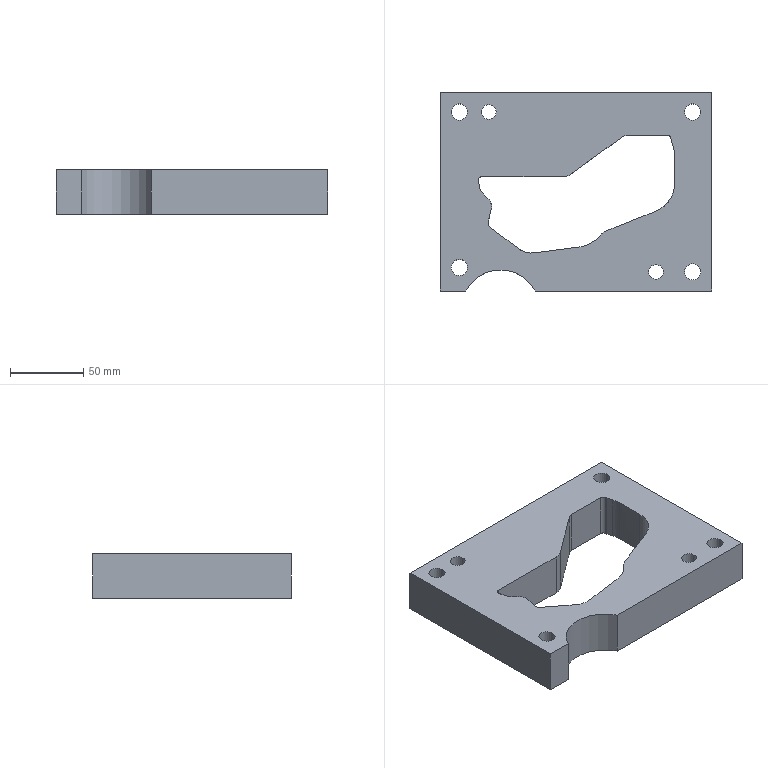Part | STEP file | 209_id714_x_t | 1 solid | 55 faces | box 185 x 135 x 30 mm | volume 513788 mm3 | cylinder 19 | plane 18 | other 18 | commonest cylinder face diameters 11 x6 5 x4 17 x4 10 x3 20 x1 53 x1